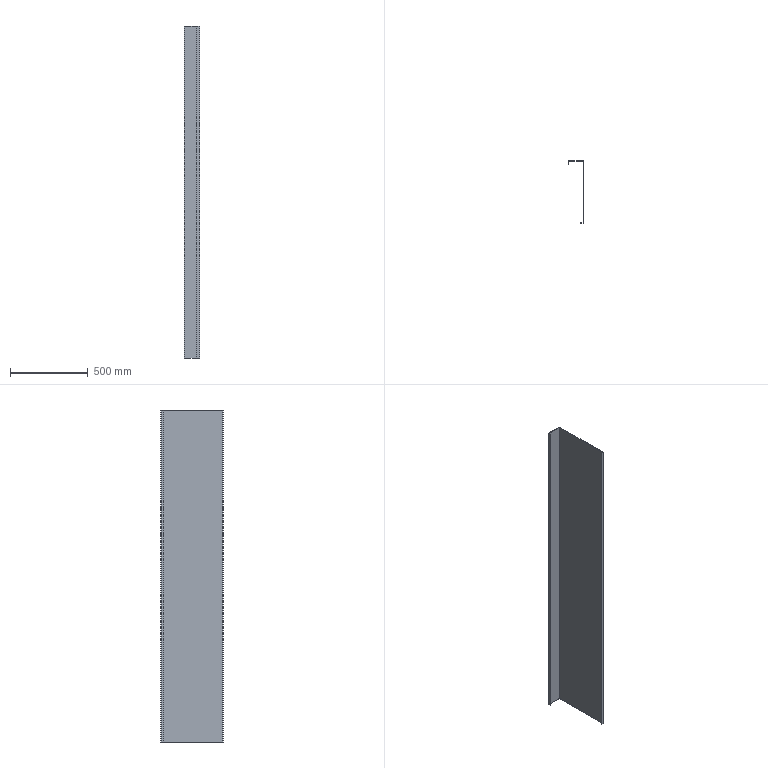Part | SolidWorks | features Extrusion 1, FlatPattern 1, SheetMetal 1, SolidToSheetMetal 1 | 1 solid | 30 faces | box 100 x 400 x 2130 mm | volume 2258384 mm3 | plane 24 | cylinder 6 | commonest cylinder face diameters 4 x3 8 x3
STEP:
#1=CARTESIAN_POINT('',(4.,18.,2130.));
#2=VERTEX_POINT('',#1);
#3=CARTESIAN_POINT('',(4.,20.,2130.));
#4=VERTEX_POINT('',#3);
#5=CARTESIAN_POINT('',(4.,20.,2130.));
#6=DIRECTION('',(0.,1.,0.));
#7=VECTOR('',#6,1000.);
#8=LINE('',#5,#7);
#9=EDGE_CURVE('',#2,#4,#8,.T.);
#10=ORIENTED_EDGE('',*,*,#9,.F.);
#11=CARTESIAN_POINT('',(96.,18.,2130.));
#12=VERTEX_POINT('',#11);
#13=CARTESIAN_POINT('',(100.,18.,2130.));
#14=DIRECTION('',(-1.,0.,0.));
#15=VECTOR('',#14,1000.);
#16=LINE('',#13,#15);
#17=EDGE_CURVE('',#12,#2,#16,.T.);
#18=ORIENTED_EDGE('',*,*,#17,.F.);
#19=CARTESIAN_POINT('',(96.,20.,2130.));
#20=VERTEX_POINT('',#19);
#21=CARTESIAN_POINT('',(96.,20.,2130.));
#22=DIRECTION('',(0.,1.,0.));
#23=VECTOR('',#22,1000.);
#24=LINE('',#21,#23);
#25=EDGE_CURVE('',#12,#20,#24,.T.);
#26=ORIENTED_EDGE('',*,*,#25,.T.);
#27=CARTESIAN_POINT('',(100.,20.,2130.));
#28=DIRECTION('',(-1.,0.,0.));
#29=VECTOR('',#28,1000.);
#30=LINE('',#27,#29);
#31=EDGE_CURVE('',#20,#4,#30,.T.);
#32=ORIENTED_EDGE('',*,*,#31,.T.);
#33=EDGE_LOOP('',(#10,#18,#26,#32));
#34=FACE_OUTER_BOUND('',#33,.T.);
#35=CARTESIAN_POINT('',(100.,20.,2130.));
#36=DIRECTION('',(0.,0.,1.));
#37=DIRECTION('',(-1.,0.,0.));
#38=AXIS2_PLACEMENT_3D('',#35,#36,#37);
#39=PLANE('',#38);
#40=ADVANCED_FACE('',(#34),#39,.T.);
#41=ORIENTED_EDGE('',*,*,#25,.F.);
#42=CARTESIAN_POINT('',(98.,16.,2130.));
#43=VERTEX_POINT('',#42);
#44=CARTESIAN_POINT('',(96.,16.,2130.));
#45=DIRECTION('',(0.,0.,-1.));
#46=DIRECTION('',(-1.,0.,0.));
#47=AXIS2_PLACEMENT_3D('',#44,#45,#46);
#48=CIRCLE('',#47,2.);
#49=EDGE_CURVE('',#12,#43,#48,.T.);
#50=ORIENTED_EDGE('',*,*,#49,.T.);
#51=CARTESIAN_POINT('',(100.,16.,2130.));
#52=VERTEX_POINT('',#51);
#53=CARTESIAN_POINT('',(100.,16.,2130.));
#54=DIRECTION('',(1.,0.,0.));
#55=VECTOR('',#54,1000.);
#56=LINE('',#53,#55);
#57=EDGE_CURVE('',#43,#52,#56,.T.);
#58=ORIENTED_EDGE('',*,*,#57,.T.);
#59=CARTESIAN_POINT('',(96.,16.,2130.));
#60=DIRECTION('',(0.,0.,-1.));
#61=DIRECTION('',(1.,0.,0.));
#62=AXIS2_PLACEMENT_3D('',#59,#60,#61);
#63=CIRCLE('',#62,4.);
#64=EDGE_CURVE('',#20,#52,#63,.T.);
#65=ORIENTED_EDGE('',*,*,#64,.F.);
#66=EDGE_LOOP('',(#41,#50,#58,#65));
#67=FACE_OUTER_BOUND('',#66,.T.);
#68=CARTESIAN_POINT('',(96.,16.,2130.));
#69=DIRECTION('',(0.,0.,-1.));
#70=DIRECTION('',(-1.,0.,0.));
#71=AXIS2_PLACEMENT_3D('',#68,#69,#70);
#72=PLANE('',#71);
#73=ADVANCED_FACE('',(#67),#72,.F.);
#74=ORIENTED_EDGE('',*,*,#57,.F.);
#75=CARTESIAN_POINT('',(98.,-376.,2130.));
#76=VERTEX_POINT('',#75);
#77=CARTESIAN_POINT('',(98.,-380.,2130.));
#78=DIRECTION('',(0.,1.,0.));
#79=VECTOR('',#78,1000.);
#80=LINE('',#77,#79);
#81=EDGE_CURVE('',#76,#43,#80,.T.);
#82=ORIENTED_EDGE('',*,*,#81,.F.);
#83=CARTESIAN_POINT('',(100.,-376.,2130.));
#84=VERTEX_POINT('',#83);
#85=CARTESIAN_POINT('',(100.,-376.,2130.));
#86=DIRECTION('',(1.,0.,0.));
#87=VECTOR('',#86,1000.);
#88=LINE('',#85,#87);
#89=EDGE_CURVE('',#76,#84,#88,.T.);
#90=ORIENTED_EDGE('',*,*,#89,.T.);
#91=CARTESIAN_POINT('',(100.,-380.,2130.));
#92=DIRECTION('',(0.,1.,0.));
#93=VECTOR('',#92,1000.);
#94=LINE('',#91,#93);
#95=EDGE_CURVE('',#84,#52,#94,.T.);
#96=ORIENTED_EDGE('',*,*,#95,.T.);
#97=EDGE_LOOP('',(#74,#82,#90,#96));
#98=FACE_OUTER_BOUND('',#97,.T.);
#99=CARTESIAN_POINT('',(100.,-380.,2130.));
#100=DIRECTION('',(0.,0.,1.));
#101=DIRECTION('',(0.,1.,0.));
#102=AXIS2_PLACEMENT_3D('',#99,#100,#101);
#103=PLANE('',#102);
#104=ADVANCED_FACE('',(#98),#103,.T.);
#105=ORIENTED_EDGE('',*,*,#89,.F.);
#106=CARTESIAN_POINT('',(96.,-378.,2130.));
#107=VERTEX_POINT('',#106);
#108=CARTESIAN_POINT('',(96.,-376.,2130.));
#109=DIRECTION('',(0.,0.,-1.));
#110=DIRECTION('',(-1.,0.,0.));
#111=AXIS2_PLACEMENT_3D('',#108,#109,#110);
#112=CIRCLE('',#111,2.);
#113=EDGE_CURVE('',#76,#107,#112,.T.);
#114=ORIENTED_EDGE('',*,*,#113,.T.);
#115=CARTESIAN_POINT('',(96.,-380.,2130.));
#116=VERTEX_POINT('',#115);
#117=CARTESIAN_POINT('',(96.,-380.,2130.));
#118=DIRECTION('',(0.,-1.,0.));
#119=VECTOR('',#118,1000.);
#120=LINE('',#117,#119);
#121=EDGE_CURVE('',#107,#116,#120,.T.);
#122=ORIENTED_EDGE('',*,*,#121,.T.);
#123=CARTESIAN_POINT('',(96.,-376.,2130.));
#124=DIRECTION('',(0.,0.,-1.));
#125=DIRECTION('',(1.,0.,0.));
#126=AXIS2_PLACEMENT_3D('',#123,#124,#125);
#127=CIRCLE('',#126,4.);
#128=EDGE_CURVE('',#84,#116,#127,.T.);
#129=ORIENTED_EDGE('',*,*,#128,.F.);
#130=EDGE_LOOP('',(#105,#114,#122,#129));
#131=FACE_OUTER_BOUND('',#130,.T.);
#132=CARTESIAN_POINT('',(96.,-376.,2130.));
#133=DIRECTION('',(0.,0.,-1.));
#134=DIRECTION('',(-1.,0.,0.));
#135=AXIS2_PLACEMENT_3D('',#132,#133,#134);
#136=PLANE('',#135);
#137=ADVANCED_FACE('',(#131),#136,.F.);
#138=ORIENTED_EDGE('',*,*,#121,.F.);
#139=CARTESIAN_POINT('',(80.,-378.,2130.));
#140=VERTEX_POINT('',#139);
#141=CARTESIAN_POINT('',(80.,-378.,2130.));
#142=DIRECTION('',(1.,0.,0.));
#143=VECTOR('',#142,1000.);
#144=LINE('',#141,#143);
#145=EDGE_CURVE('',#140,#107,#144,.T.);
#146=ORIENTED_EDGE('',*,*,#145,.F.);
#147=CARTESIAN_POINT('',(80.,-380.,2130.));
#148=VERTEX_POINT('',#147);
#149=CARTESIAN_POINT('',(80.,-380.,2130.));
#150=DIRECTION('',(0.,-1.,0.));
#151=VECTOR('',#150,1000.);
#152=LINE('',#149,#151);
#153=EDGE_CURVE('',#140,#148,#152,.T.);
#154=ORIENTED_EDGE('',*,*,#153,.T.);
#155=CARTESIAN_POINT('',(80.,-380.,2130.));
#156=DIRECTION('',(1.,0.,0.));
#157=VECTOR('',#156,1000.);
#158=LINE('',#155,#157);
#159=EDGE_CURVE('',#148,#116,#158,.T.);
#160=ORIENTED_EDGE('',*,*,#159,.T.);
#161=EDGE_LOOP('',(#138,#146,#154,#160));
#162=FACE_OUTER_BOUND('',#161,.T.);
#163=CARTESIAN_POINT('',(80.,-380.,2130.));
#164=DIRECTION('',(0.,0.,1.));
#165=DIRECTION('',(1.,0.,0.));
#166=AXIS2_PLACEMENT_3D('',#163,#164,#165);
#167=PLANE('',#166);
#168=ADVANCED_FACE('',(#162),#167,.T.);
#169=ORIENTED_EDGE('',*,*,#153,.F.);
#170=CARTESIAN_POINT('',(80.,-378.,0.));
#171=VERTEX_POINT('',#170);
#172=CARTESIAN_POINT('',(80.,-378.,2130.));
#173=DIRECTION('',(0.,0.,-1.));
#174=VECTOR('',#173,1000.);
#175=LINE('',#172,#174);
#176=EDGE_CURVE('',#140,#171,#175,.T.);
#177=ORIENTED_EDGE('',*,*,#176,.T.);
#178=CARTESIAN_POINT('',(80.,-380.,0.));
#179=VERTEX_POINT('',#178);
#180=CARTESIAN_POINT('',(80.,-380.,0.));
#181=DIRECTION('',(0.,-1.,0.));
#182=VECTOR('',#181,1000.);
#183=LINE('',#180,#182);
#184=EDGE_CURVE('',#171,#179,#183,.T.);
#185=ORIENTED_EDGE('',*,*,#184,.T.);
#186=CARTESIAN_POINT('',(80.,-380.,2130.));
#187=DIRECTION('',(0.,0.,-1.));
#188=VECTOR('',#187,1000.);
#189=LINE('',#186,#188);
#190=EDGE_CURVE('',#148,#179,#189,.T.);
#191=ORIENTED_EDGE('',*,*,#190,.F.);
#192=EDGE_LOOP('',(#169,#177,#185,#191));
#193=FACE_OUTER_BOUND('',#192,.T.);
#194=CARTESIAN_POINT('',(80.,-380.,2130.));
#195=DIRECTION('',(1.,0.,0.));
#196=DIRECTION('',(0.,0.,-1.));
#197=AXIS2_PLACEMENT_3D('',#194,#195,#196);
#198=PLANE('',#197);
#199=ADVANCED_FACE('',(#193),#198,.F.);
#200=ORIENTED_EDGE('',*,*,#184,.F.);
#201=CARTESIAN_POINT('',(96.,-378.,0.));
#202=VERTEX_POINT('',#201);
#203=CARTESIAN_POINT('',(80.,-378.,0.));
#204=DIRECTION('',(1.,0.,0.));
#205=VECTOR('',#204,1000.);
#206=LINE('',#203,#205);
#207=EDGE_CURVE('',#171,#202,#206,.T.);
#208=ORIENTED_EDGE('',*,*,#207,.T.);
#209=CARTESIAN_POINT('',(96.,-380.,0.));
#210=VERTEX_POINT('',#209);
#211=CARTESIAN_POINT('',(96.,-380.,0.));
#212=DIRECTION('',(0.,-1.,0.));
#213=VECTOR('',#212,1000.);
#214=LINE('',#211,#213);
#215=EDGE_CURVE('',#202,#210,#214,.T.);
#216=ORIENTED_EDGE('',*,*,#215,.T.);
#217=CARTESIAN_POINT('',(80.,-380.,0.));
#218=DIRECTION('',(1.,0.,0.));
#219=VECTOR('',#218,1000.);
#220=LINE('',#217,#219);
#221=EDGE_CURVE('',#179,#210,#220,.T.);
#222=ORIENTED_EDGE('',*,*,#221,.F.);
#223=EDGE_LOOP('',(#200,#208,#216,#222));
#224=FACE_OUTER_BOUND('',#223,.T.);
#225=CARTESIAN_POINT('',(80.,-380.,0.));
#226=DIRECTION('',(0.,0.,1.));
#227=DIRECTION('',(1.,0.,0.));
#228=AXIS2_PLACEMENT_3D('',#225,#226,#227);
#229=PLANE('',#228);
#230=ADVANCED_FACE('',(#224),#229,.F.);
#231=ORIENTED_EDGE('',*,*,#215,.F.);
#232=CARTESIAN_POINT('',(98.,-376.,0.));
#233=VERTEX_POINT('',#232);
#234=CARTESIAN_POINT('',(96.,-376.,0.));
#235=DIRECTION('',(0.,0.,1.));
#236=DIRECTION('',(-1.,0.,0.));
#237=AXIS2_PLACEMENT_3D('',#234,#235,#236);
#238=CIRCLE('',#237,2.);
#239=EDGE_CURVE('',#202,#233,#238,.T.);
#240=ORIENTED_EDGE('',*,*,#239,.T.);
#241=CARTESIAN_POINT('',(100.,-376.,0.));
#242=VERTEX_POINT('',#241);
#243=CARTESIAN_POINT('',(100.,-376.,0.));
#244=DIRECTION('',(1.,0.,0.));
#245=VECTOR('',#244,1000.);
#246=LINE('',#243,#245);
#247=EDGE_CURVE('',#233,#242,#246,.T.);
#248=ORIENTED_EDGE('',*,*,#247,.T.);
#249=CARTESIAN_POINT('',(96.,-376.,0.));
#250=DIRECTION('',(0.,0.,1.));
#251=DIRECTION('',(-1.,0.,0.));
#252=AXIS2_PLACEMENT_3D('',#249,#250,#251);
#253=CIRCLE('',#252,4.);
#254=EDGE_CURVE('',#210,#242,#253,.T.);
#255=ORIENTED_EDGE('',*,*,#254,.F.);
#256=EDGE_LOOP('',(#231,#240,#248,#255));
#257=FACE_OUTER_BOUND('',#256,.T.);
#258=CARTESIAN_POINT('',(96.,-376.,0.));
#259=DIRECTION('',(0.,0.,1.));
#260=DIRECTION('',(1.,0.,0.));
#261=AXIS2_PLACEMENT_3D('',#258,#259,#260);
#262=PLANE('',#261);
#263=ADVANCED_FACE('',(#257),#262,.F.);
#264=ORIENTED_EDGE('',*,*,#247,.F.);
#265=CARTESIAN_POINT('',(98.,16.,0.));
#266=VERTEX_POINT('',#265);
#267=CARTESIAN_POINT('',(98.,-380.,0.));
#268=DIRECTION('',(0.,1.,0.));
#269=VECTOR('',#268,1000.);
#270=LINE('',#267,#269);
#271=EDGE_CURVE('',#233,#266,#270,.T.);
#272=ORIENTED_EDGE('',*,*,#271,.T.);
#273=CARTESIAN_POINT('',(100.,16.,0.));
#274=VERTEX_POINT('',#273);
#275=CARTESIAN_POINT('',(100.,16.,0.));
#276=DIRECTION('',(1.,0.,0.));
#277=VECTOR('',#276,1000.);
#278=LINE('',#275,#277);
#279=EDGE_CURVE('',#266,#274,#278,.T.);
#280=ORIENTED_EDGE('',*,*,#279,.T.);
#281=CARTESIAN_POINT('',(100.,-380.,0.));
#282=DIRECTION('',(0.,1.,0.));
#283=VECTOR('',#282,1000.);
#284=LINE('',#281,#283);
#285=EDGE_CURVE('',#242,#274,#284,.T.);
#286=ORIENTED_EDGE('',*,*,#285,.F.);
#287=EDGE_LOOP('',(#264,#272,#280,#286));
#288=FACE_OUTER_BOUND('',#287,.T.);
#289=CARTESIAN_POINT('',(100.,-380.,0.));
#290=DIRECTION('',(0.,0.,1.));
#291=DIRECTION('',(0.,1.,0.));
#292=AXIS2_PLACEMENT_3D('',#289,#290,#291);
#293=PLANE('',#292);
#294=ADVANCED_FACE('',(#288),#293,.F.);
#295=ORIENTED_EDGE('',*,*,#279,.F.);
#296=CARTESIAN_POINT('',(96.,18.,0.));
#297=VERTEX_POINT('',#296);
#298=CARTESIAN_POINT('',(96.,16.,0.));
#299=DIRECTION('',(0.,0.,1.));
#300=DIRECTION('',(-1.,0.,0.));
#301=AXIS2_PLACEMENT_3D('',#298,#299,#300);
#302=CIRCLE('',#301,2.);
#303=EDGE_CURVE('',#266,#297,#302,.T.);
#304=ORIENTED_EDGE('',*,*,#303,.T.);
#305=CARTESIAN_POINT('',(96.,20.,0.));
#306=VERTEX_POINT('',#305);
#307=CARTESIAN_POINT('',(96.,20.,0.));
#308=DIRECTION('',(0.,1.,0.));
#309=VECTOR('',#308,1000.);
#310=LINE('',#307,#309);
#311=EDGE_CURVE('',#297,#306,#310,.T.);
#312=ORIENTED_EDGE('',*,*,#311,.T.);
#313=CARTESIAN_POINT('',(96.,16.,0.));
#314=DIRECTION('',(0.,0.,1.));
#315=DIRECTION('',(-1.,0.,0.));
#316=AXIS2_PLACEMENT_3D('',#313,#314,#315);
#317=CIRCLE('',#316,4.);
#318=EDGE_CURVE('',#274,#306,#317,.T.);
#319=ORIENTED_EDGE('',*,*,#318,.F.);
#320=EDGE_LOOP('',(#295,#304,#312,#319));
#321=FACE_OUTER_BOUND('',#320,.T.);
#322=CARTESIAN_POINT('',(96.,16.,0.));
#323=DIRECTION('',(0.,0.,1.));
#324=DIRECTION('',(1.,0.,0.));
#325=AXIS2_PLACEMENT_3D('',#322,#323,#324);
#326=PLANE('',#325);
#327=ADVANCED_FACE('',(#321),#326,.F.);
#328=ORIENTED_EDGE('',*,*,#311,.F.);
#329=CARTESIAN_POINT('',(4.,18.,0.));
#330=VERTEX_POINT('',#329);
#331=CARTESIAN_POINT('',(100.,18.,0.));
#332=DIRECTION('',(-1.,0.,0.));
#333=VECTOR('',#332,1000.);
#334=LINE('',#331,#333);
#335=EDGE_CURVE('',#297,#330,#334,.T.);
#336=ORIENTED_EDGE('',*,*,#335,.T.);
#337=CARTESIAN_POINT('',(4.,20.,0.));
#338=VERTEX_POINT('',#337);
#339=CARTESIAN_POINT('',(4.,20.,0.));
#340=DIRECTION('',(0.,1.,0.));
#341=VECTOR('',#340,1000.);
#342=LINE('',#339,#341);
#343=EDGE_CURVE('',#330,#338,#342,.T.);
#344=ORIENTED_EDGE('',*,*,#343,.T.);
#345=CARTESIAN_POINT('',(100.,20.,0.));
#346=DIRECTION('',(-1.,0.,0.));
#347=VECTOR('',#346,1000.);
#348=LINE('',#345,#347);
#349=EDGE_CURVE('',#306,#338,#348,.T.);
#350=ORIENTED_EDGE('',*,*,#349,.F.);
#351=EDGE_LOOP('',(#328,#336,#344,#350));
#352=FACE_OUTER_BOUND('',#351,.T.);
#353=CARTESIAN_POINT('',(100.,20.,0.));
#354=DIRECTION('',(0.,0.,1.));
#355=DIRECTION('',(-1.,0.,0.));
#356=AXIS2_PLACEMENT_3D('',#353,#354,#355);
#357=PLANE('',#356);
#358=ADVANCED_FACE('',(#352),#357,.F.);
#359=ORIENTED_EDGE('',*,*,#343,.F.);
#360=CARTESIAN_POINT('',(2.,16.,0.));
#361=VERTEX_POINT('',#360);
#362=CARTESIAN_POINT('',(4.,16.,0.));
#363=DIRECTION('',(0.,0.,1.));
#364=DIRECTION('',(-1.,0.,0.));
#365=AXIS2_PLACEMENT_3D('',#362,#363,#364);
#366=CIRCLE('',#365,2.);
#367=EDGE_CURVE('',#330,#361,#366,.T.);
#368=ORIENTED_EDGE('',*,*,#367,.T.);
#369=CARTESIAN_POINT('',(0.,16.,0.));
#370=VERTEX_POINT('',#369);
#371=CARTESIAN_POINT('',(0.,16.,0.));
#372=DIRECTION('',(-1.,0.,0.));
#373=VECTOR('',#372,1000.);
#374=LINE('',#371,#373);
#375=EDGE_CURVE('',#361,#370,#374,.T.);
#376=ORIENTED_EDGE('',*,*,#375,.T.);
#377=CARTESIAN_POINT('',(4.,16.,0.));
#378=DIRECTION('',(0.,0.,1.));
#379=DIRECTION('',(-1.,0.,0.));
#380=AXIS2_PLACEMENT_3D('',#377,#378,#379);
#381=CIRCLE('',#380,4.);
#382=EDGE_CURVE('',#338,#370,#381,.T.);
#383=ORIENTED_EDGE('',*,*,#382,.F.);
#384=EDGE_LOOP('',(#359,#368,#376,#383));
#385=FACE_OUTER_BOUND('',#384,.T.);
#386=CARTESIAN_POINT('',(4.,16.,0.));
#387=DIRECTION('',(0.,0.,1.));
#388=DIRECTION('',(1.,0.,0.));
#389=AXIS2_PLACEMENT_3D('',#386,#387,#388);
#390=PLANE('',#389);
#391=ADVANCED_FACE('',(#385),#390,.F.);
#392=ORIENTED_EDGE('',*,*,#375,.F.);
#393=CARTESIAN_POINT('',(2.,0.,0.));
#394=VERTEX_POINT('',#393);
#395=CARTESIAN_POINT('',(2.,20.,0.));
#396=DIRECTION('',(0.,-1.,0.));
#397=VECTOR('',#396,1000.);
#398=LINE('',#395,#397);
#399=EDGE_CURVE('',#361,#394,#398,.T.);
#400=ORIENTED_EDGE('',*,*,#399,.T.);
#401=CARTESIAN_POINT('',(0.,0.,0.));
#402=VERTEX_POINT('',#401);
#403=CARTESIAN_POINT('',(0.,0.,0.));
#404=DIRECTION('',(-1.,0.,0.));
#405=VECTOR('',#404,1000.);
#406=LINE('',#403,#405);
#407=EDGE_CURVE('',#394,#402,#406,.T.);
#408=ORIENTED_EDGE('',*,*,#407,.T.);
#409=CARTESIAN_POINT('',(0.,20.,0.));
#410=DIRECTION('',(0.,-1.,0.));
#411=VECTOR('',#410,1000.);
#412=LINE('',#409,#411);
#413=EDGE_CURVE('',#370,#402,#412,.T.);
#414=ORIENTED_EDGE('',*,*,#413,.F.);
#415=EDGE_LOOP('',(#392,#400,#408,#414));
#416=FACE_OUTER_BOUND('',#415,.T.);
#417=CARTESIAN_POINT('',(0.,20.,0.));
#418=DIRECTION('',(0.,0.,1.));
#419=DIRECTION('',(0.,-1.,0.));
#420=AXIS2_PLACEMENT_3D('',#417,#418,#419);
#421=PLANE('',#420);
#422=ADVANCED_FACE('',(#416),#421,.F.);
#423=ORIENTED_EDGE('',*,*,#407,.F.);
#424=CARTESIAN_POINT('',(2.,0.,2130.));
#425=VERTEX_POINT('',#424);
#426=CARTESIAN_POINT('',(2.,0.,2130.));
#427=DIRECTION('',(0.,0.,-1.));
#428=VECTOR('',#427,1000.);
#429=LINE('',#426,#428);
#430=EDGE_CURVE('',#425,#394,#429,.T.);
#431=ORIENTED_EDGE('',*,*,#430,.F.);
#432=CARTESIAN_POINT('',(0.,0.,2130.));
#433=VERTEX_POINT('',#432);
#434=CARTESIAN_POINT('',(0.,0.,2130.));
#435=DIRECTION('',(-1.,0.,0.));
#436=VECTOR('',#435,1000.);
#437=LINE('',#434,#436);
#438=EDGE_CURVE('',#425,#433,#437,.T.);
#439=ORIENTED_EDGE('',*,*,#438,.T.);
#440=CARTESIAN_POINT('',(0.,0.,2130.));
#441=DIRECTION('',(0.,0.,-1.));
#442=VECTOR('',#441,1000.);
#443=LINE('',#440,#442);
#444=EDGE_CURVE('',#433,#402,#443,.T.);
#445=ORIENTED_EDGE('',*,*,#444,.T.);
#446=EDGE_LOOP('',(#423,#431,#439,#445));
#447=FACE_OUTER_BOUND('',#446,.T.);
#448=CARTESIAN_POINT('',(0.,0.,2130.));
#449=DIRECTION('',(0.,-1.,0.));
#450=DIRECTION('',(0.,0.,-1.));
#451=AXIS2_PLACEMENT_3D('',#448,#449,#450);
#452=PLANE('',#451);
#453=ADVANCED_FACE('',(#447),#452,.T.);
#454=ORIENTED_EDGE('',*,*,#438,.F.);
#455=CARTESIAN_POINT('',(2.,16.,2130.));
#456=VERTEX_POINT('',#455);
#457=CARTESIAN_POINT('',(2.,20.,2130.));
#458=DIRECTION('',(0.,-1.,0.));
#459=VECTOR('',#458,1000.);
#460=LINE('',#457,#459);
#461=EDGE_CURVE('',#456,#425,#460,.T.);
#462=ORIENTED_EDGE('',*,*,#461,.F.);
#463=CARTESIAN_POINT('',(0.,16.,2130.));
#464=VERTEX_POINT('',#463);
#465=CARTESIAN_POINT('',(0.,16.,2130.));
#466=DIRECTION('',(-1.,0.,0.));
#467=VECTOR('',#466,1000.);
#468=LINE('',#465,#467);
#469=EDGE_CURVE('',#456,#464,#468,.T.);
#470=ORIENTED_EDGE('',*,*,#469,.T.);
#471=CARTESIAN_POINT('',(0.,20.,2130.));
#472=DIRECTION('',(0.,-1.,0.));
#473=VECTOR('',#472,1000.);
#474=LINE('',#471,#473);
#475=EDGE_CURVE('',#464,#433,#474,.T.);
#476=ORIENTED_EDGE('',*,*,#475,.T.);
#477=EDGE_LOOP('',(#454,#462,#470,#476));
#478=FACE_OUTER_BOUND('',#477,.T.);
#479=CARTESIAN_POINT('',(0.,20.,2130.));
#480=DIRECTION('',(0.,0.,1.));
#481=DIRECTION('',(0.,-1.,0.));
#482=AXIS2_PLACEMENT_3D('',#479,#480,#481);
#483=PLANE('',#482);
#484=ADVANCED_FACE('',(#478),#483,.T.);
#485=CARTESIAN_POINT('',(4.,16.,2130.));
#486=DIRECTION('',(0.,0.,-1.));
#487=DIRECTION('',(-1.,0.,0.));
#488=AXIS2_PLACEMENT_3D('',#485,#486,#487);
#489=CIRCLE('',#488,2.);
#490=EDGE_CURVE('',#456,#2,#489,.T.);
#491=ORIENTED_EDGE('',*,*,#490,.T.);
#492=ORIENTED_EDGE('',*,*,#9,.T.);
#493=CARTESIAN_POINT('',(4.,16.,2130.));
#494=DIRECTION('',(0.,0.,-1.));
#495=DIRECTION('',(1.,0.,0.));
#496=AXIS2_PLACEMENT_3D('',#493,#494,#495);
#497=CIRCLE('',#496,4.);
#498=EDGE_CURVE('',#464,#4,#497,.T.);
#499=ORIENTED_EDGE('',*,*,#498,.F.);
#500=ORIENTED_EDGE('',*,*,#469,.F.);
#501=EDGE_LOOP('',(#491,#492,#499,#500));
#502=FACE_OUTER_BOUND('',#501,.T.);
#503=CARTESIAN_POINT('',(4.,16.,2130.));
#504=DIRECTION('',(0.,0.,-1.));
#505=DIRECTION('',(-1.,0.,0.));
#506=AXIS2_PLACEMENT_3D('',#503,#504,#505);
#507=PLANE('',#506);
#508=ADVANCED_FACE('',(#502),#507,.F.);
#509=ORIENTED_EDGE('',*,*,#475,.F.);
#510=CARTESIAN_POINT('',(0.,16.,2130.));
#511=DIRECTION('',(0.,0.,-1.));
#512=VECTOR('',#511,1000.);
#513=LINE('',#510,#512);
#514=EDGE_CURVE('',#464,#370,#513,.T.);
#515=ORIENTED_EDGE('',*,*,#514,.T.);
#516=ORIENTED_EDGE('',*,*,#413,.T.);
#517=ORIENTED_EDGE('',*,*,#444,.F.);
#518=EDGE_LOOP('',(#509,#515,#516,#517));
#519=FACE_OUTER_BOUND('',#518,.T.);
#520=CARTESIAN_POINT('',(0.,20.,2130.));
#521=DIRECTION('',(1.,0.,0.));
#522=DIRECTION('',(0.,0.,-1.));
#523=AXIS2_PLACEMENT_3D('',#520,#521,#522);
#524=PLANE('',#523);
#525=ADVANCED_FACE('',(#519),#524,.F.);
#526=ORIENTED_EDGE('',*,*,#31,.F.);
#527=CARTESIAN_POINT('',(96.,20.,2130.));
#528=DIRECTION('',(0.,0.,-1.));
#529=VECTOR('',#528,1000.);
#530=LINE('',#527,#529);
#531=EDGE_CURVE('',#20,#306,#530,.T.);
#532=ORIENTED_EDGE('',*,*,#531,.T.);
#533=ORIENTED_EDGE('',*,*,#349,.T.);
#534=CARTESIAN_POINT('',(4.,20.,2130.));
#535=DIRECTION('',(0.,0.,1.));
#536=VECTOR('',#535,1000.);
#537=LINE('',#534,#536);
#538=EDGE_CURVE('',#338,#4,#537,.T.);
#539=ORIENTED_EDGE('',*,*,#538,.T.);
#540=EDGE_LOOP('',(#526,#532,#533,#539));
#541=FACE_OUTER_BOUND('',#540,.T.);
#542=CARTESIAN_POINT('',(100.,20.,2130.));
#543=DIRECTION('',(0.,-1.,0.));
#544=DIRECTION('',(0.,0.,-1.));
#545=AXIS2_PLACEMENT_3D('',#542,#543,#544);
#546=PLANE('',#545);
#547=ADVANCED_FACE('',(#541),#546,.F.);
#548=ORIENTED_EDGE('',*,*,#221,.T.);
#549=CARTESIAN_POINT('',(96.,-380.,2130.));
#550=DIRECTION('',(0.,0.,1.));
#551=VECTOR('',#550,1000.);
#552=LINE('',#549,#551);
#553=EDGE_CURVE('',#210,#116,#552,.T.);
#554=ORIENTED_EDGE('',*,*,#553,.T.);
#555=ORIENTED_EDGE('',*,*,#159,.F.);
#556=ORIENTED_EDGE('',*,*,#190,.T.);
#557=EDGE_LOOP('',(#548,#554,#555,#556));
#558=FACE_OUTER_BOUND('',#557,.T.);
#559=CARTESIAN_POINT('',(80.,-380.,2130.));
#560=DIRECTION('',(0.,1.,0.));
#561=DIRECTION('',(0.,0.,1.));
#562=AXIS2_PLACEMENT_3D('',#559,#560,#561);
#563=PLANE('',#562);
#564=ADVANCED_FACE('',(#558),#563,.F.);
#565=ORIENTED_EDGE('',*,*,#285,.T.);
#566=CARTESIAN_POINT('',(100.,16.,2130.));
#567=DIRECTION('',(0.,0.,1.));
#568=VECTOR('',#567,1000.);
#569=LINE('',#566,#568);
#570=EDGE_CURVE('',#274,#52,#569,.T.);
#571=ORIENTED_EDGE('',*,*,#570,.T.);
#572=ORIENTED_EDGE('',*,*,#95,.F.);
#573=CARTESIAN_POINT('',(100.,-376.,2130.));
#574=DIRECTION('',(0.,0.,-1.));
#575=VECTOR('',#574,1000.);
#576=LINE('',#573,#575);
#577=EDGE_CURVE('',#84,#242,#576,.T.);
#578=ORIENTED_EDGE('',*,*,#577,.T.);
#579=EDGE_LOOP('',(#565,#571,#572,#578));
#580=FACE_OUTER_BOUND('',#579,.T.);
#581=CARTESIAN_POINT('',(100.,-380.,2130.));
#582=DIRECTION('',(-1.,0.,0.));
#583=DIRECTION('',(0.,0.,1.));
#584=AXIS2_PLACEMENT_3D('',#581,#582,#583);
#585=PLANE('',#584);
#586=ADVANCED_FACE('',(#580),#585,.F.);
#587=ORIENTED_EDGE('',*,*,#498,.T.);
#588=ORIENTED_EDGE('',*,*,#538,.F.);
#589=ORIENTED_EDGE('',*,*,#382,.T.);
#590=ORIENTED_EDGE('',*,*,#514,.F.);
#591=EDGE_LOOP('',(#587,#588,#589,#590));
#592=FACE_OUTER_BOUND('',#591,.T.);
#593=CARTESIAN_POINT('',(4.,16.,2130.));
#594=DIRECTION('',(0.,0.,-1.));
#595=DIRECTION('',(-1.,0.,0.));
#596=AXIS2_PLACEMENT_3D('',#593,#594,#595);
#597=CYLINDRICAL_SURFACE('',#596,4.);
#598=ADVANCED_FACE('',(#592),#597,.T.);
#599=ORIENTED_EDGE('',*,*,#128,.T.);
#600=ORIENTED_EDGE('',*,*,#553,.F.);
#601=ORIENTED_EDGE('',*,*,#254,.T.);
#602=ORIENTED_EDGE('',*,*,#577,.F.);
#603=EDGE_LOOP('',(#599,#600,#601,#602));
#604=FACE_OUTER_BOUND('',#603,.T.);
#605=CARTESIAN_POINT('',(96.,-376.,2130.));
#606=DIRECTION('',(0.,0.,-1.));
#607=DIRECTION('',(-1.,0.,0.));
#608=AXIS2_PLACEMENT_3D('',#605,#606,#607);
#609=CYLINDRICAL_SURFACE('',#608,4.);
#610=ADVANCED_FACE('',(#604),#609,.T.);
#611=ORIENTED_EDGE('',*,*,#64,.T.);
#612=ORIENTED_EDGE('',*,*,#570,.F.);
#613=ORIENTED_EDGE('',*,*,#318,.T.);
#614=ORIENTED_EDGE('',*,*,#531,.F.);
#615=EDGE_LOOP('',(#611,#612,#613,#614));
#616=FACE_OUTER_BOUND('',#615,.T.);
#617=CARTESIAN_POINT('',(96.,16.,2130.));
#618=DIRECTION('',(0.,0.,-1.));
#619=DIRECTION('',(-1.,0.,0.));
#620=AXIS2_PLACEMENT_3D('',#617,#618,#619);
#621=CYLINDRICAL_SURFACE('',#620,4.);
#622=ADVANCED_FACE('',(#616),#621,.T.);
#623=ORIENTED_EDGE('',*,*,#461,.T.);
#624=ORIENTED_EDGE('',*,*,#430,.T.);
#625=ORIENTED_EDGE('',*,*,#399,.F.);
#626=CARTESIAN_POINT('',(2.,16.,2130.));
#627=DIRECTION('',(0.,0.,-1.));
#628=VECTOR('',#627,1000.);
#629=LINE('',#626,#628);
#630=EDGE_CURVE('',#456,#361,#629,.T.);
#631=ORIENTED_EDGE('',*,*,#630,.F.);
#632=EDGE_LOOP('',(#623,#624,#625,#631));
#633=FACE_OUTER_BOUND('',#632,.T.);
#634=CARTESIAN_POINT('',(2.,20.,2130.));
#635=DIRECTION('',(1.,0.,0.));
#636=DIRECTION('',(0.,0.,-1.));
#637=AXIS2_PLACEMENT_3D('',#634,#635,#636);
#638=PLANE('',#637);
#639=ADVANCED_FACE('',(#633),#638,.T.);
#640=ORIENTED_EDGE('',*,*,#17,.T.);
#641=CARTESIAN_POINT('',(4.,18.,2130.));
#642=DIRECTION('',(0.,0.,1.));
#643=VECTOR('',#642,1000.);
#644=LINE('',#641,#643);
#645=EDGE_CURVE('',#330,#2,#644,.T.);
#646=ORIENTED_EDGE('',*,*,#645,.F.);
#647=ORIENTED_EDGE('',*,*,#335,.F.);
#648=CARTESIAN_POINT('',(96.,18.,2130.));
#649=DIRECTION('',(0.,0.,-1.));
#650=VECTOR('',#649,1000.);
#651=LINE('',#648,#650);
#652=EDGE_CURVE('',#12,#297,#651,.T.);
#653=ORIENTED_EDGE('',*,*,#652,.F.);
#654=EDGE_LOOP('',(#640,#646,#647,#653));
#655=FACE_OUTER_BOUND('',#654,.T.);
#656=CARTESIAN_POINT('',(100.,18.,2130.));
#657=DIRECTION('',(0.,-1.,0.));
#658=DIRECTION('',(0.,0.,-1.));
#659=AXIS2_PLACEMENT_3D('',#656,#657,#658);
#660=PLANE('',#659);
#661=ADVANCED_FACE('',(#655),#660,.T.);
#662=ORIENTED_EDGE('',*,*,#207,.F.);
#663=ORIENTED_EDGE('',*,*,#176,.F.);
#664=ORIENTED_EDGE('',*,*,#145,.T.);
#665=CARTESIAN_POINT('',(96.,-378.,2130.));
#666=DIRECTION('',(0.,0.,1.));
#667=VECTOR('',#666,1000.);
#668=LINE('',#665,#667);
#669=EDGE_CURVE('',#202,#107,#668,.T.);
#670=ORIENTED_EDGE('',*,*,#669,.F.);
#671=EDGE_LOOP('',(#662,#663,#664,#670));
#672=FACE_OUTER_BOUND('',#671,.T.);
#673=CARTESIAN_POINT('',(80.,-378.,2130.));
#674=DIRECTION('',(0.,1.,0.));
#675=DIRECTION('',(0.,0.,1.));
#676=AXIS2_PLACEMENT_3D('',#673,#674,#675);
#677=PLANE('',#676);
#678=ADVANCED_FACE('',(#672),#677,.T.);
#679=ORIENTED_EDGE('',*,*,#271,.F.);
#680=CARTESIAN_POINT('',(98.,-376.,2130.));
#681=DIRECTION('',(0.,0.,-1.));
#682=VECTOR('',#681,1000.);
#683=LINE('',#680,#682);
#684=EDGE_CURVE('',#76,#233,#683,.T.);
#685=ORIENTED_EDGE('',*,*,#684,.F.);
#686=ORIENTED_EDGE('',*,*,#81,.T.);
#687=CARTESIAN_POINT('',(98.,16.,2130.));
#688=DIRECTION('',(0.,0.,1.));
#689=VECTOR('',#688,1000.);
#690=LINE('',#687,#689);
#691=EDGE_CURVE('',#266,#43,#690,.T.);
#692=ORIENTED_EDGE('',*,*,#691,.F.);
#693=EDGE_LOOP('',(#679,#685,#686,#692));
#694=FACE_OUTER_BOUND('',#693,.T.);
#695=CARTESIAN_POINT('',(98.,-380.,2130.));
#696=DIRECTION('',(-1.,0.,0.));
#697=DIRECTION('',(0.,0.,1.));
#698=AXIS2_PLACEMENT_3D('',#695,#696,#697);
#699=PLANE('',#698);
#700=ADVANCED_FACE('',(#694),#699,.T.);
#701=ORIENTED_EDGE('',*,*,#490,.F.);
#702=ORIENTED_EDGE('',*,*,#630,.T.);
#703=ORIENTED_EDGE('',*,*,#367,.F.);
#704=ORIENTED_EDGE('',*,*,#645,.T.);
#705=EDGE_LOOP('',(#701,#702,#703,#704));
#706=FACE_OUTER_BOUND('',#705,.T.);
#707=CARTESIAN_POINT('',(4.,16.,2130.));
#708=DIRECTION('',(0.,0.,-1.));
#709=DIRECTION('',(-1.,0.,0.));
#710=AXIS2_PLACEMENT_3D('',#707,#708,#709);
#711=CYLINDRICAL_SURFACE('',#710,2.);
#712=ADVANCED_FACE('',(#706),#711,.F.);
#713=ORIENTED_EDGE('',*,*,#113,.F.);
#714=ORIENTED_EDGE('',*,*,#684,.T.);
#715=ORIENTED_EDGE('',*,*,#239,.F.);
#716=ORIENTED_EDGE('',*,*,#669,.T.);
#717=EDGE_LOOP('',(#713,#714,#715,#716));
#718=FACE_OUTER_BOUND('',#717,.T.);
#719=CARTESIAN_POINT('',(96.,-376.,2130.));
#720=DIRECTION('',(0.,0.,-1.));
#721=DIRECTION('',(-1.,0.,0.));
#722=AXIS2_PLACEMENT_3D('',#719,#720,#721);
#723=CYLINDRICAL_SURFACE('',#722,2.);
#724=ADVANCED_FACE('',(#718),#723,.F.);
#725=ORIENTED_EDGE('',*,*,#49,.F.);
#726=ORIENTED_EDGE('',*,*,#652,.T.);
#727=ORIENTED_EDGE('',*,*,#303,.F.);
#728=ORIENTED_EDGE('',*,*,#691,.T.);
#729=EDGE_LOOP('',(#725,#726,#727,#728));
#730=FACE_OUTER_BOUND('',#729,.T.);
#731=CARTESIAN_POINT('',(96.,16.,2130.));
#732=DIRECTION('',(0.,0.,-1.));
#733=DIRECTION('',(-1.,0.,0.));
#734=AXIS2_PLACEMENT_3D('',#731,#732,#733);
#735=CYLINDRICAL_SURFACE('',#734,2.);
#736=ADVANCED_FACE('',(#730),#735,.F.);
#737=CLOSED_SHELL('',(#40,#73,#104,#137,#168,#199,#230,#263,#294,#327,#358,#391,#422,#453,#484,#508,#525,#547,#564,#586,#598,#610,#622,#639,#661,#678,#700,#712,#724,#736));
#738=MANIFOLD_SOLID_BREP('',#737);
#739=CARTESIAN_POINT('',(0.,0.,0.));
#740=DIRECTION('',(0.,0.,1.));
#741=DIRECTION('',(1.,0.,0.));
#742=AXIS2_PLACEMENT_3D('',#739,#740,#741);
#743=(LENGTH_UNIT()NAMED_UNIT(*)SI_UNIT(.MILLI.,.METRE.));
#744=UNCERTAINTY_MEASURE_WITH_UNIT(LENGTH_MEASURE(0.00001),#743,'','');
#745=(NAMED_UNIT(*)PLANE_ANGLE_UNIT()SI_UNIT($,.RADIAN.));
#746=(NAMED_UNIT(*)SI_UNIT($,.STERADIAN.)SOLID_ANGLE_UNIT());
#747=(GEOMETRIC_REPRESENTATION_CONTEXT(3)GLOBAL_UNCERTAINTY_ASSIGNED_CONTEXT((#744))GLOBAL_UNIT_ASSIGNED_CONTEXT((#743,#745,#746))REPRESENTATION_CONTEXT('',''));
#748=ADVANCED_BREP_SHAPE_REPRESENTATION('',(#738,#742),#747);